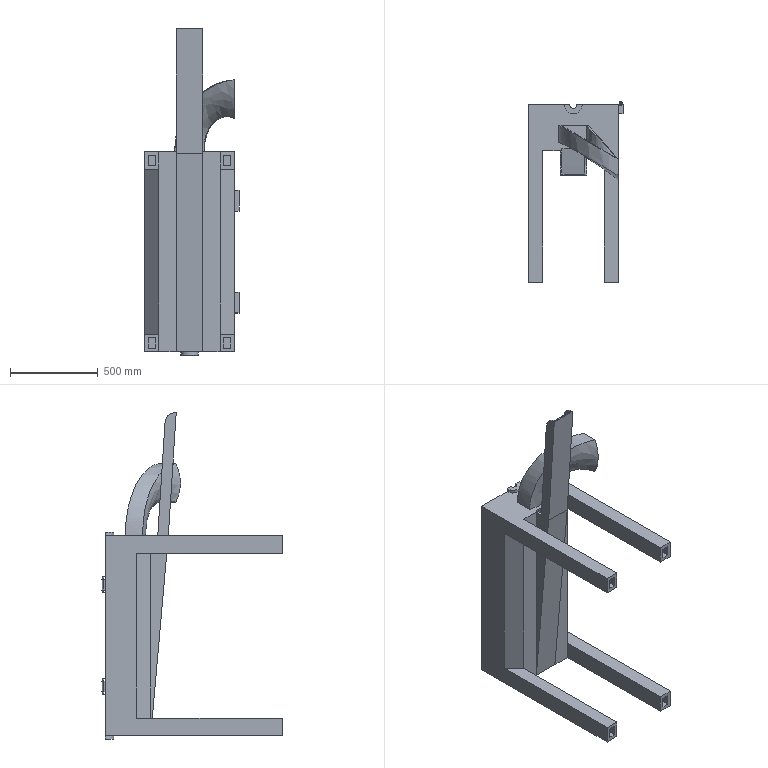Part | SolidWorks | 1 solid | 650 faces | box 540 x 1030 x 1860 mm | volume 48317416 mm3 | cylinder 504 | plane 137 | spline 9 | commonest cylinder face diameters 30 x484 10 x8 20 x2 40 x2 68 x2 100 x2